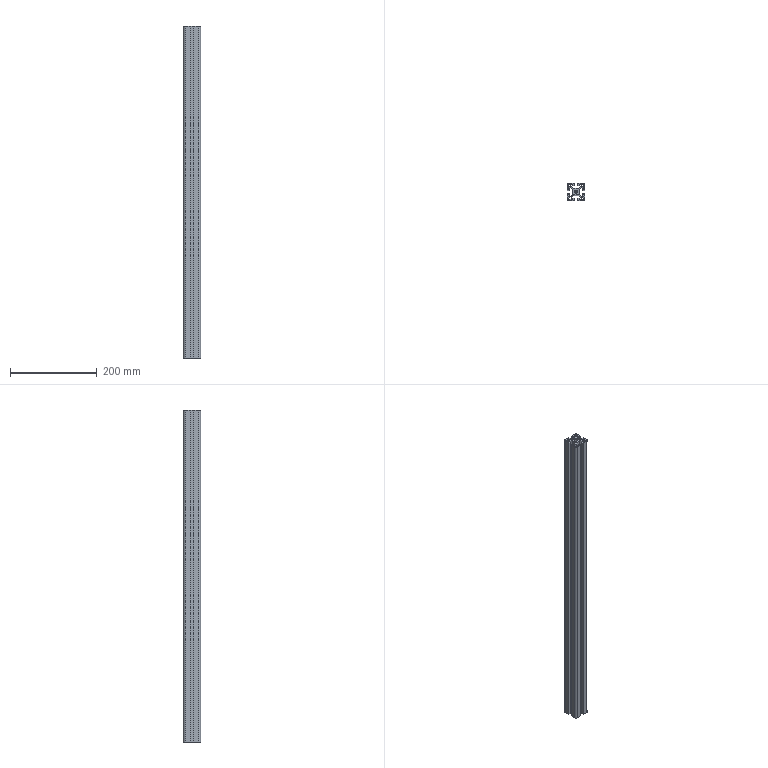Part | STEP file | 4040-765 | 1 solid | 88 faces | box 40 x 40 x 765 mm | volume 538519 mm3 | plane 78 | cylinder 10 | commonest cylinder face diameters 4 x4 10 x4 6.8 x2